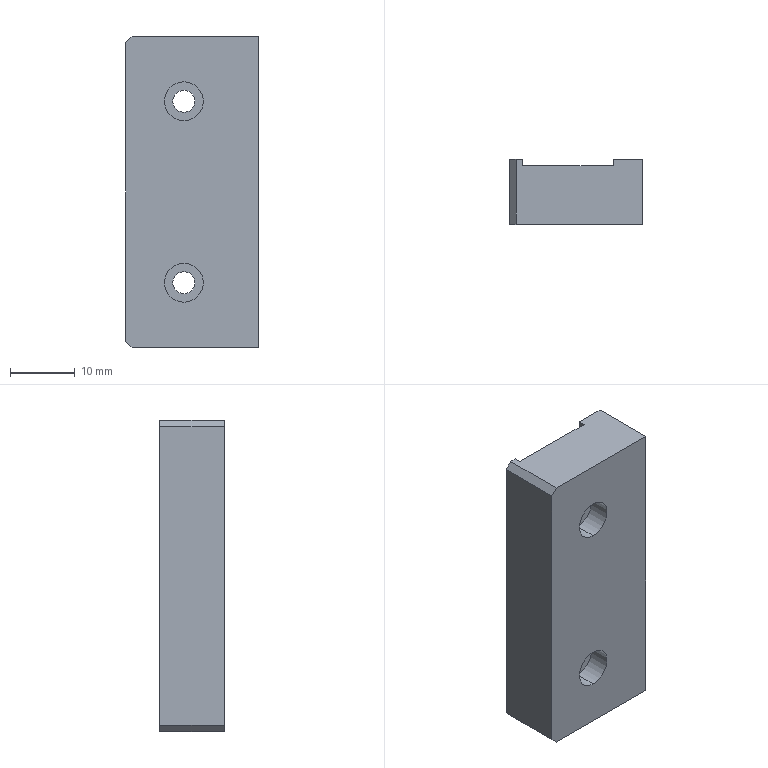Part | STEP file | 2059 Cylinder press block A | 1 solid | 34 faces | box 20.5 x 10 x 48 mm | volume 8560 mm3 | cylinder 14 | plane 14 | cone 6 | commonest cylinder face diameters 3.3 x6 3.4 x4 6 x4